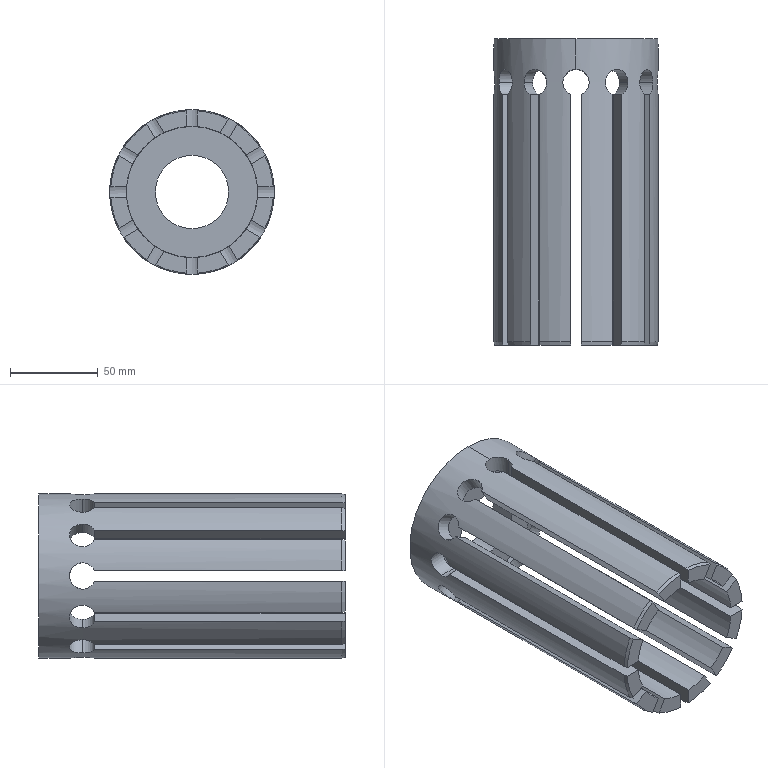Part | STEP file | PN_0005 Press head | 1 solid | 104 faces | box 94 x 175 x 94 mm | volume 368252 mm3 | cylinder 48 | plane 38 | cone 18 | commonest cylinder face diameters 15 x36 4.2 x6 42 x2 75 x2 94 x2